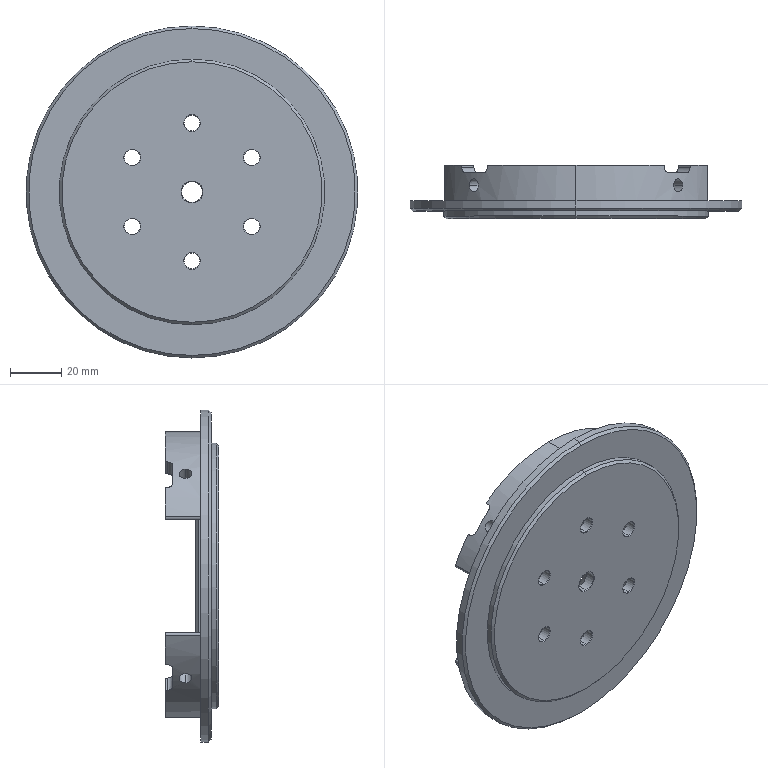Part | NX | features BREP 1 | 1 solid | 125 faces | box 130 x 20.9 x 130 mm | volume 102210 mm3 | cylinder 57 | cone 35 | plane 33 | commonest cylinder face diameters 2 x12 6.2 x12 4 x8 5 x8 100 x4 113.2 x4